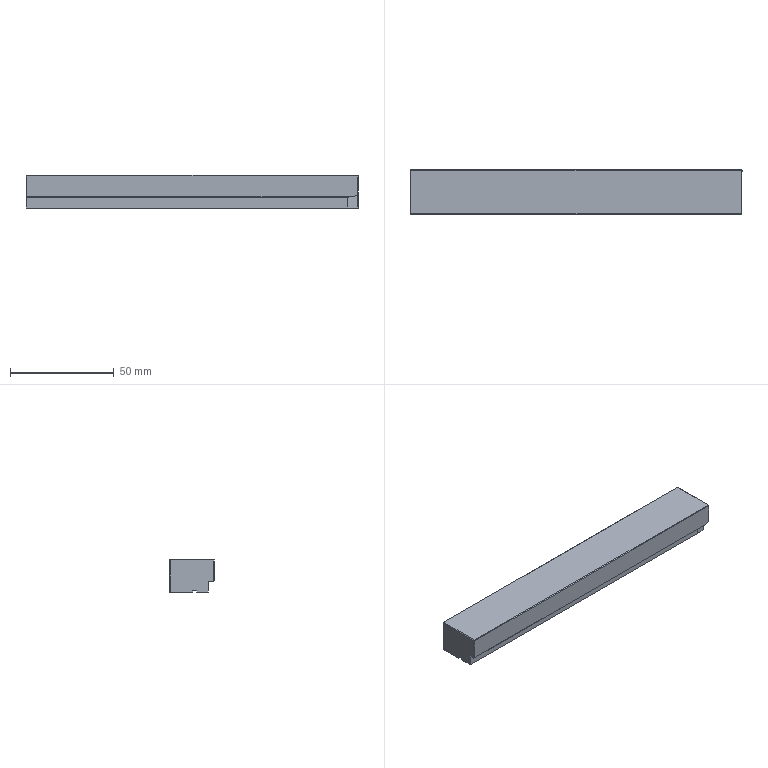Part | NX | 1 solid | 79 faces | box 159.75 x 21.5 x 16 mm | volume 51547 mm3 | plane 31 | cone 24 | cylinder 24 | commonest cylinder face diameters 2.5 x12 3.3 x12